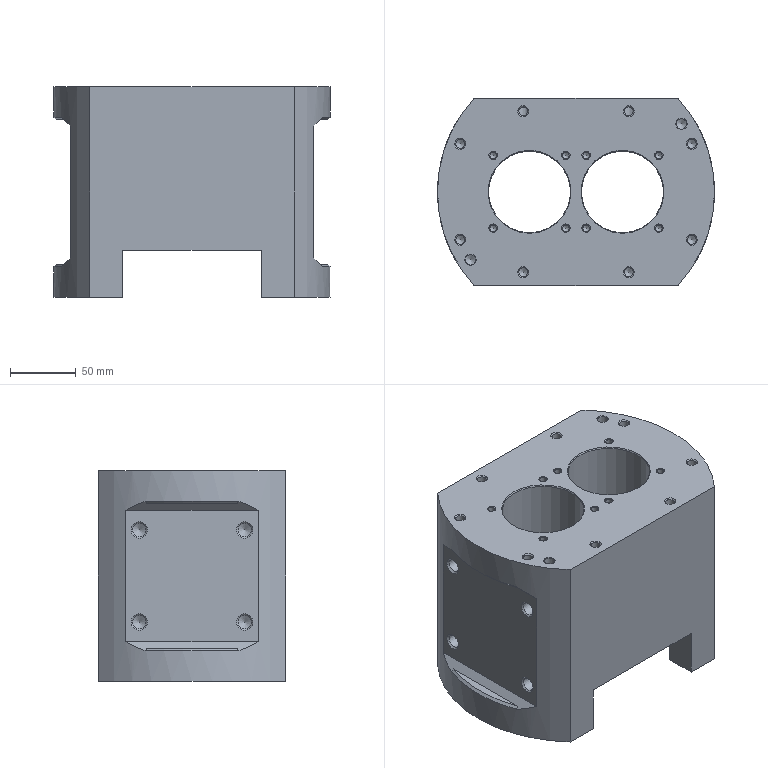NC program | NX | posted with a generic post | part box 210 x 142 x 160 mm
Lines 3328 to 4199 of 4199:
(FLOOR_WALL_2_COPY , TOOL : D10JING)
N6648 T11 M6
N6650 G54
N6652 G17 G0 G90 X-47.5 Y79. B0. C0. S5000 M3
N6654 G43 Z30. H11
N6656 Z-1.5
N6658 G94 G1 Z-4.5 F500.
N6660 Y76.
N6662 Y44.478 F1200.
N6664 X-50.809 Y43.289
N6666 G3 X-50.809 Y-43.289 R46.
N6668 G1 X-47.5 Y-44.478
N6670 Y-76.
N6672 Y-79.
N6674 Z-1.5
N6676 G0 Z30.
N6678 X47.5
N6680 Z-1.5
N6682 G1 Z-4.5 F500.
N6684 Y-76.
N6686 Y-44.478 F1200.
N6688 X50.809 Y-43.289
N6690 G3 X50.809 Y43.289 R46.
N6692 G1 X47.5 Y44.478
N6694 Y76.
N6696 Y79.
N6698 Z-1.5
N6700 G0 Z30.
N6702 X-47.5
N6704 Z-6.
N6706 G1 Z-9. F500.
N6708 Y76.
N6710 Y44.478 F1200.
N6712 X-50.809 Y43.289
N6714 G3 X-50.809 Y-43.289 R46.
N6716 G1 X-47.5 Y-44.478
N6718 Y-76.
N6720 Y-79.
N6722 Z-6.
N6724 G0 Z30.
N6726 X47.5
N6728 Z-6.
N6730 G1 Z-9. F500.
N6732 Y-76.
N6734 Y-44.478 F1200.
N6736 X50.809 Y-43.289
N6738 G3 X50.809 Y43.289 R46.
N6740 G1 X47.5 Y44.478
N6742 Y76.
N6744 Y79.
N6746 Z-6.
N6748 G0 Z30.
N6750 X-47.5
N6752 Z-10.5
N6754 G1 Z-13.5 F500.
N6756 Y76.
N6758 Y44.478 F1200.
N6760 X-50.809 Y43.289
N6762 G3 X-50.809 Y-43.289 R46.
N6764 G1 X-47.5 Y-44.478
N6766 Y-76.
N6768 Y-79.
N6770 Z-10.5
N6772 G0 Z30.
N6774 X47.5
N6776 Z-10.5
N6778 G1 Z-13.5 F500.
N6780 Y-76.
N6782 Y-44.478 F1200.
N6784 X50.809 Y-43.289
N6786 G3 X50.809 Y43.289 R46.
N6788 G1 X47.5 Y44.478
N6790 Y76.
N6792 Y79.
N6794 Z-10.5
N6796 G0 Z30.
N6798 X-47.5
N6800 Z-15.
N6802 G1 Z-18. F500.
N6804 Y76.
N6806 Y44.478 F1200.
N6808 X-50.809 Y43.289
N6810 G3 X-50.809 Y-43.289 R46.
N6812 G1 X-47.5 Y-44.478
N6814 Y-76.
N6816 Y-79.
N6818 Z-15.
N6820 G0 Z30.
N6822 X47.5
N6824 Z-15.
N6826 G1 Z-18. F500.
N6828 Y-76.
N6830 Y-44.478 F1200.
N6832 X50.809 Y-43.289
N6834 G3 X50.809 Y43.289 R46.
N6836 G1 X47.5 Y44.478
N6838 Y76.
N6840 Y79.
N6842 Z-15.
N6844 G0 Z30.
N6846 X-47.5
N6848 Z-19.5
N6850 G1 Z-22.5 F500.
N6852 Y76.
N6854 Y44.478 F1200.
N6856 X-50.809 Y43.289
N6858 G3 X-50.809 Y-43.289 R46.
N6860 G1 X-47.5 Y-44.478
N6862 Y-76.
N6864 Y-79.
N6866 Z-19.5
N6868 G0 Z30.
N6870 X47.5
N6872 Z-19.5
N6874 G1 Z-22.5 F500.
N6876 Y-76.
N6878 Y-44.478 F1200.
N6880 X50.809 Y-43.289
N6882 G3 X50.809 Y43.289 R46.
N6884 G1 X47.5 Y44.478
N6886 Y76.
N6888 Y79.
N6890 Z-19.5
N6892 G0 Z30.
N6894 X-47.5
N6896 Z-24.
N6898 G1 Z-27. F500.
N6900 Y76.
N6902 Y44.478 F1200.
N6904 X-50.809 Y43.289
N6906 G3 X-50.809 Y-43.289 R46.
N6908 G1 X-47.5 Y-44.478
N6910 Y-76.
N6912 Y-79.
N6914 Z-24.
N6916 G0 Z30.
N6918 X47.5
N6920 Z-24.
N6922 G1 Z-27. F500.
N6924 Y-76.
N6926 Y-44.478 F1200.
N6928 X50.809 Y-43.289
N6930 G3 X50.809 Y43.289 R46.
N6932 G1 X47.5 Y44.478
N6934 Y76.
N6936 Y79.
N6938 Z-24.
N6940 G0 Z30.
N6942 X-47.5
N6944 Z-28.5
N6946 G1 Z-31.5 F500.
N6948 Y76.
N6950 Y44.478 F1200.
N6952 X-50.809 Y43.289
N6954 G3 X-50.809 Y-43.289 R46.
N6956 G1 X-47.5 Y-44.478
N6958 Y-76.
N6960 Y-79.
N6962 Z-28.5
N6964 G0 Z30.
N6966 X47.5
N6968 Z-28.5
N6970 G1 Z-31.5 F500.
N6972 Y-76.
N6974 Y-44.478 F1200.
N6976 X50.809 Y-43.289
N6978 G3 X50.809 Y43.289 R46.
N6980 G1 X47.5 Y44.478
N6982 Y76.
N6984 Y79.
N6986 Z-28.5
N6988 G0 Z30.
N6990 X-47.5
N6992 Z-33.
N6994 G1 Z-36. F500.
N6996 Y76.
N6998 Y44.478 F1200.
N7000 X-50.809 Y43.289
N7002 G3 X-50.809 Y-43.289 R46.
N7004 G1 X-47.5 Y-44.478
N7006 Y-76.
N7008 Y-79.
N7010 Z-33.
N7012 G0 Z30.
N7014 X47.5
N7016 Z-33.
N7018 G1 Z-36. F500.
N7020 Y-76.
N7022 Y-44.478 F1200.
N7024 X50.809 Y-43.289
N7026 G3 X50.809 Y43.289 R46.
N7028 G1 X47.5 Y44.478
N7030 Y76.
N7032 Y79.
N7034 Z-33.
N7036 G0 Z30.
(FLOOR_WALL_2 , TOOL : D10JING)
N7038 X-80.75 Y-0.024
N7040 Z-30.
N7042 G95 G1 Y0.049 Z-30.019 F3.
N7044 Y-0.049 Z-30.046
N7046 Y0.049 Z-30.072
N7048 Y-0.049 Z-30.099
N7050 Y0.049 Z-30.125
N7052 Y-0.049 Z-30.151
N7054 Y0.049 Z-30.178
N7056 Y-0.049 Z-30.204
N7058 Y0.049 Z-30.23
N7060 Y-0.049 Z-30.257
N7062 Y0.049 Z-30.283
N7064 Y-0.049 Z-30.309
N7066 Y0.049 Z-30.336
N7068 Y-0.049 Z-30.362
N7070 Y0.049 Z-30.388
N7072 Y-0.049 Z-30.415
N7074 Y0.049 Z-30.441
N7076 Y-0.049 Z-30.467
N7078 Y0.049 Z-30.494
N7080 Y-0.049 Z-30.52
N7082 Y0.049 Z-30.546
N7084 Y-0.049 Z-30.573
N7086 Y0.049 Z-30.599
N7088 Y-0.049 Z-30.625
N7090 Y0.049 Z-30.652
N7092 Y-0.049 Z-30.678
N7094 Y0.049 Z-30.704
N7096 Y-0.049 Z-30.731
N7098 Y0.049 Z-30.757
N7100 Y-0.049 Z-30.784
N7102 Y0.049 Z-30.81
N7104 Y-0.049 Z-30.836
N7106 Y0.049 Z-30.863
N7108 Y-0.049 Z-30.889
N7110 Y0.049 Z-30.915
N7112 Y-0.049 Z-30.942
N7114 Y0.049 Z-30.968
N7116 Y-0.049 Z-30.994
N7118 Y0.049 Z-31.021
N7120 Y-0.049 Z-31.047
N7122 Y0.049 Z-31.073
N7124 Y-0.049 Z-31.1
N7126 Y0.049 Z-31.126
N7128 Y-0.049 Z-31.152
N7130 Y0.049 Z-31.179
N7132 Y-0.049 Z-31.205
N7134 Y0.049 Z-31.231
N7136 Y-0.049 Z-31.258
N7138 Y0.049 Z-31.284
N7140 Y-0.049 Z-31.31
N7142 Y0.049 Z-31.337
N7144 Y-0.049 Z-31.363
N7146 Y0.049 Z-31.389
N7148 Y-0.049 Z-31.416
N7150 Y0.049 Z-31.442
N7152 Y-0.049 Z-31.469
N7154 Y0.049 Z-31.495
N7156 Y-0.049 Z-31.521
N7158 Y0.049 Z-31.548
N7160 Y-0.049 Z-31.574
N7162 Y0.049 Z-31.6
N7164 Y-0.049 Z-31.627
N7166 Y0.049 Z-31.653
N7168 Y-0.049 Z-31.679
N7170 Y0.049 Z-31.706
N7172 Y-0.049 Z-31.732
N7174 Y0.049 Z-31.758
N7176 Y-0.049 Z-31.785
N7178 Y0.049 Z-31.811
N7180 Y-0.049 Z-31.837
N7182 Y0.049 Z-31.864
N7184 Y-0.049 Z-31.89
N7186 Y0.049 Z-31.916
N7188 Y-0.049 Z-31.943
N7190 Y0.049 Z-31.969
N7192 Y-0.049 Z-31.995
N7194 Y0.049 Z-32.022
N7196 Y-0.049 Z-32.048
N7198 Y0.049 Z-32.074
N7200 Y-0.049 Z-32.101
N7202 Y0.049 Z-32.127
N7204 Y-0.049 Z-32.154
N7206 Y0.049 Z-32.18
N7208 Y-0.049 Z-32.206
N7210 Y0.049 Z-32.233
N7212 Y-0.049 Z-32.259
N7214 Y0.049 Z-32.285
N7216 Y-0.049 Z-32.312
N7218 Y0.049 Z-32.338
N7220 Y-0.049 Z-32.364
N7222 Y0.049 Z-32.391
N7224 Y-0.049 Z-32.417
N7226 Y0.049 Z-32.443
N7228 Y-0.049 Z-32.47
N7230 Y0.049 Z-32.496
N7232 Y-0.049 Z-32.522
N7234 Y0.049 Z-32.549
N7236 Y-0.049 Z-32.575
N7238 Y0.049 Z-32.601
N7240 Y-0.049 Z-32.628
N7242 Y0.049 Z-32.654
N7244 Y-0.049 Z-32.68
N7246 Y0.049 Z-32.707
N7248 Y-0.049 Z-32.733
N7250 Y0.049 Z-32.759
N7252 Y-0.049 Z-32.786
N7254 Y0.049 Z-32.812
N7256 Y-0.049 Z-32.839
N7258 Y0.049 Z-32.865
N7260 Y-0.049 Z-32.891
N7262 Y0.049 Z-32.918
N7264 Y-0.049 Z-32.944
N7266 Y0.049 Z-32.97
N7268 Y-0.049 Z-32.997
N7270 Y0.049 Z-33.023
N7272 Y-0.049 Z-33.049
N7274 Y0.049 Z-33.076
N7276 Y-0.049 Z-33.102
N7278 Y0.049 Z-33.128
N7280 Y-0.049 Z-33.155
N7282 Y0.049 Z-33.181
N7284 Y-0.049 Z-33.207
N7286 Y0.049 Z-33.234
N7288 Y-0.049 Z-33.26
N7290 Y0.049 Z-33.286
N7292 Y-0.049 Z-33.313
N7294 Y0.049 Z-33.339
N7296 Y-0.049 Z-33.365
N7298 Y0.049 Z-33.392
N7300 Y-0.049 Z-33.418
N7302 Y0.049 Z-33.444
N7304 Y-0.049 Z-33.471
N7306 Y0.049 Z-33.497
N7308 Y-0.049 Z-33.523
N7310 Y0.049 Z-33.55
N7312 Y-0.049 Z-33.576
N7314 Y0.049 Z-33.603
N7316 Y-0.049 Z-33.629
N7318 Y0.049 Z-33.655
N7320 Y-0.049 Z-33.682
N7322 Y0.049 Z-33.708
N7324 Y-0.049 Z-33.734
N7326 Y0.049 Z-33.761
N7328 Y-0.049 Z-33.787
N7330 Y0.049 Z-33.813
N7332 Y-0.049 Z-33.84
N7334 Y0.049 Z-33.866
N7336 Y-0.049 Z-33.892
N7338 Y0.049 Z-33.919
N7340 Y-0.049 Z-33.945
N7342 Y0.049 Z-33.971
N7344 Y-0.049 Z-33.998
N7346 Y0.049 Z-34.024
N7348 Y-0.049 Z-34.05
N7350 Y0.049 Z-34.077
N7352 Y-0.049 Z-34.103
N7354 Y0.049 Z-34.129
N7356 Y-0.049 Z-34.156
N7358 Y0.049 Z-34.182
N7360 Y-0.049 Z-34.208
N7362 Y0.049 Z-34.235
N7364 Y-0.049 Z-34.261
N7366 Y0.049 Z-34.288
N7368 Y-0.049 Z-34.314
N7370 Y0.049 Z-34.34
N7372 Y-0.049 Z-34.367
N7374 Y0.049 Z-34.393
N7376 Y-0.049 Z-34.419
N7378 Y0.049 Z-34.446
N7380 Y-0.049 Z-34.472
N7382 Y0.049 Z-34.498
N7384 Y-0.049 Z-34.525
N7386 Y0.049 Z-34.551
N7388 Y-0.049 Z-34.577
N7390 Y0.049 Z-34.604
N7392 Y-0.049 Z-34.63
N7394 Y0.049 Z-34.656
N7396 Y-0.049 Z-34.683
N7398 Y0.049 Z-34.709
N7400 Y-0.049 Z-34.735
N7402 Y0.049 Z-34.762
N7404 Y-0.049 Z-34.788
N7406 Y0.049 Z-34.814
N7408 Y-0.049 Z-34.841
N7410 Y0.049 Z-34.867
N7412 Y-0.049 Z-34.893
N7414 Y0.049 Z-34.92
N7416 Y-0.049 Z-34.946
N7418 Y0.049 Z-34.973
N7420 Y-0.049 Z-34.999
N7422 Y0.049 Z-35.025
N7424 Y-0.049 Z-35.052
N7426 Y0.049 Z-35.078
N7428 Y-0.049 Z-35.104
N7430 Y0.049 Z-35.131
N7432 Y-0.049 Z-35.157
N7434 Y0.049 Z-35.183
N7436 Y-0.049 Z-35.21
N7438 Y0.049 Z-35.236
N7440 Y-0.049 Z-35.262
N7442 Y0.049 Z-35.289
N7444 Y-0.049 Z-35.315
N7446 Y0.049 Z-35.341
N7448 Y-0.049 Z-35.368
N7450 Y0.049 Z-35.394
N7452 Y-0.049 Z-35.42
N7454 Y0.049 Z-35.447
N7456 Y-0.049 Z-35.473
N7458 Y0.049 Z-35.499
N7460 Y-0.049 Z-35.526
N7462 Y0.049 Z-35.552
N7464 Y-0.049 Z-35.578
N7466 Y0.049 Z-35.605
N7468 Y-0.049 Z-35.631
N7470 Y0.049 Z-35.658
N7472 Y-0.049 Z-35.684
N7474 Y0.049 Z-35.71
N7476 Y-0.049 Z-35.737
N7478 Y0.049 Z-35.763
N7480 Y-0.049 Z-35.789
N7482 Y0.049 Z-35.816
N7484 Y-0.049 Z-35.842
N7486 Y0.049 Z-35.868
N7488 Y-0.049 Z-35.895
N7490 Y0.049 Z-35.921
N7492 Y-0.049 Z-35.947
N7494 Y0.049 Z-35.974
N7496 Y-0.049 Z-36.
N7498 G94 Y0.049 F1200.
N7500 G2 X-75.856 Y20.528 R45.5
N7502 G1 Y-20.528
N7504 G3 X-70.962 Y-28.194 R45.5
N7506 G1 Y28.194
N7508 G2 X-66.068 Y33.474 R45.5
N7510 G1 Y-33.474
N7512 G3 X-61.174 Y-37.392 R45.5
N7514 G1 Y37.392
N7516 G2 X-56.28 Y40.348 R45.5
N7518 G1 Y-40.348
N7520 G3 X-51.386 Y-42.543 R45.5
N7522 G1 Y42.543
N7524 G2 X-50.64 Y42.818 R45.5
N7526 G1 X-47.331 Y44.008
N7528 G3 X-47. Y44.478 R0.5
N7530 G1 Y76.
N7532 X-46.492
N7534 Y-76.
N7536 X-41.598
N7538 Y76.
N7540 X-36.705
N7542 Y-76.
N7544 X-31.811
N7546 Y76.
N7548 X-26.917
N7550 Y-76.
N7552 X-22.023
N7554 Y76.
N7556 X-17.129
N7558 Y-76.
N7560 X-12.235
N7562 Y76.
N7564 X-7.341
N7566 Y-76.
N7568 X-2.447
N7570 Y76.
N7572 X2.447
N7574 Y-76.
N7576 X7.341
N7578 Y76.
N7580 X12.235
N7582 Y-76.
N7584 X17.129
N7586 Y76.
N7588 X22.023
N7590 Y-76.
N7592 X26.917
N7594 Y76.
N7596 X31.811
N7598 Y-76.
N7600 X36.705
N7602 Y76.
N7604 X41.598
N7606 Y-76.
N7608 X46.492
N7610 Y76.
N7612 X47.
N7614 Y44.478
N7616 G3 X47.331 Y44.008 R0.5
N7618 G1 X50.64 Y42.818
N7620 G2 X51.386 Y42.543 R45.5
N7622 G1 Y-42.543
N7624 G3 X56.28 Y-40.348 R45.5
N7626 G1 Y40.348
N7628 G2 X61.174 Y37.392 R45.5
N7630 G1 Y-37.392
N7632 G3 X66.068 Y-33.474 R45.5
N7634 G1 Y33.474
N7636 G2 X70.962 Y28.194 R45.5
N7638 G1 Y-28.194
N7640 G3 X75.856 Y-20.528 R45.5
N7642 G1 Y20.528
N7644 G2 X80.75 Y0.049 R45.5
N7646 G1 Y-0.049
N7648 Z-33.
N7650 G0 Z30.
N7652 X47.5 Y-79.
N7654 Z-33.
N7656 G95 G1 Z-36. F3.
N7658 Y-76.
N7660 G94 Y-44.478 F1200.
N7662 X50.809 Y-43.289
N7664 G3 X50.809 Y43.289 R46.
N7666 G1 X47.5 Y44.478
N7668 Y76.
N7670 Y79.
N7672 Z-33.
N7674 G0 Z30.
N7676 X-47.5
N7678 Z-33.
N7680 G95 G1 Z-36. F3.
N7682 Y76.
N7684 G94 Y44.478 F1200.
N7686 X-50.809 Y43.289
N7688 G3 X-50.809 Y-43.289 R46.
N7690 G1 X-47.5 Y-44.478
N7692 Y-76.
N7694 Y-79.
N7696 Z-33.
N7698 G0 Z30.
N7700 M5
(DRILLING_COPY_2_COPY_1 , TOOL : ZXZ)
N7702 T01 M6
N7704 G54
N7706 G17 G0 G90 X69. Y59. B0. C0. S5000 M3
N7708 G43 Z30. H1
N7710 G94 G81 G98 Z-1. F250. R3.
N7712 X82. Y47.
N7714 X62.827 Y27.577 Z-37. R-33.
N7716 X7.673
N7718 X-7.673
N7720 Y-27.577
N7722 X7.673
N7724 X35.25 Y0.
N7726 X62.827 Y-27.577
N7728 X69. Y-59. Z-1. R3.
N7730 X-69.
N7732 X-82. Y-47.
N7734 X-62.827 Y-27.577 Z-37. R-33.
N7736 X-35.25 Y0.
N7738 X-62.827 Y27.577
N7740 X-69. Y59. Z-1. R3.
N7742 G80
N7744 G0 X-69. Y59. Z30.
N7746 M5
(DRILLING_COPY_2_COPY_COPY_1_COPY_2 , TOOL : 5.2ZT)
N7748 T15 M6
N7750 G54
N7752 G17 G0 G90 X-62.827 Y-27.577 B0. C0. S2000 M3
N7754 G43 Z30. H15
N7756 G94 G83 G98 Z-57.502 F200. Q2. R-33.
N7758 Y27.577
N7760 X-7.673
N7762 X7.673
N7764 X62.827
N7766 Y-27.577
N7768 X7.673
N7770 X-7.673
N7772 G80
N7774 G0 X-7.673 Y-27.577 Z30.
N7776 M5
(DRILLING_COPY_2_COPY_COPY_1_COPY_2_COPY , TOOL : 8.5ZT)
N7778 T20 M6
N7780 G54
N7782 G17 G0 G90 X-69. Y-59. B0. C0. S2000 M3
N7784 G43 Z30. H20
N7786 G94 G83 G98 Z-32.054 F200. Q2. R3.
N7788 Y59.
N7790 X69.
N7792 Y-59.
N7794 G80
N7796 G0 X69. Y-59. Z30.
N7798 M5
(DRILLING_COPY_2_COPY_COPY_1_COPY_1_COPY_1 , TOOL : 9.8ZT)
N7800 T03 M6
N7802 G54
N7804 G17 G0 G90 X82. Y47. B0. C0. S2000 M3
N7806 G43 Z30. H3
N7808 G94 G83 G98 Z-23.004 F200. Q2. R3.
N7810 X-82. Y-47.
N7812 G80
N7814 G0 X-82. Y-47. Z30.
N7816 M5
(DRILLING_COPY_2_COPY_COPY_1_COPY_1_COPY_COPY_1 , TOOL : 10.JD)
N7818 T04 M6
N7820 G54
N7822 G17 G0 G90 X-82. Y-47. B0. C0. S1000 M3
N7824 G43 Z30. H4
N7826 G94 G85 G98 Z-20. F40. R3.
N7828 X82. Y47.
N7830 G80
N7832 G0 X82. Y47. Z30.
N7834 M5
(PLANAR_MILL_COPY_COPY_COPY_COPY_COPY_1 , TOOL : D6A45)
N7836 T07 M6
N7838 G54
N7840 G17 G0 G90 X-68.438 Y61.487 B0. C0. S7500 M3
N7842 G43 Z30. H7
N7844 Z1.5
N7846 G94 G1 Z-1.5 F1250.
N7848 X-68.234 Y62.393
N7850 G3 X-69. Y62.75 R1.
N7852 X-72.75 Y59. R3.75
N7854 X-69. Y62.75 R-3.75
N7856 X-69.766 Y62.393 R1.
N7858 G1 X-69.562 Y61.487
N7860 Z1.5
N7862 G0 Z30.
N7864 X-84.487 Y-46.438
N7866 Z1.5
N7868 G1 Z-1.5
N7870 X-85.393 Y-46.234
N7872 G3 X-85.75 Y-47. R1.
N7874 X-82. Y-50.75 R3.75
N7876 X-85.75 Y-47. R-3.75
N7878 X-85.393 Y-47.766 R1.
N7880 G1 X-84.487 Y-47.562
N7882 Z1.5
N7884 G0 Z30.
N7886 X-69.562 Y-61.487
N7888 Z1.5
N7890 G1 Z-1.5
N7892 X-69.766 Y-62.393
N7894 G3 X-69. Y-62.75 R1.
N7896 X-65.25 Y-59. R3.75
N7898 X-69. Y-62.75 R-3.75
N7900 X-68.234 Y-62.393 R1.
N7902 G1 X-68.438 Y-61.487
N7904 Z1.5
N7906 G0 Z30.
N7908 X68.438
N7910 Z1.5
N7912 G1 Z-1.5
N7914 X68.234 Y-62.393
N7916 G3 X69. Y-62.75 R1.
N7918 X72.75 Y-59. R3.75
N7920 X69. Y-62.75 R-3.75
N7922 X69.766 Y-62.393 R1.
N7924 G1 X69.562 Y-61.487
N7926 Z1.5
N7928 G0 Z30.
N7930 X84.487 Y46.438
N7932 Z1.5
N7934 G1 Z-1.5
N7936 X85.393 Y46.234
N7938 G3 X85.75 Y47. R1.
N7940 X82. Y50.75 R3.75
N7942 X85.75 Y47. R-3.75
N7944 X85.393 Y47.766 R1.
N7946 G1 X84.487 Y47.562
N7948 Z1.5
N7950 G0 Z30.
N7952 X69.562 Y61.487
N7954 Z1.5
N7956 G1 Z-1.5
N7958 X69.766 Y62.393
N7960 G3 X69. Y62.75 R1.
N7962 X65.25 Y59. R3.75
N7964 X69. Y62.75 R-3.75
N7966 X68.234 Y62.393 R1.
N7968 G1 X68.438 Y61.487
N7970 Z1.5
N7972 G0 Z30.
(PLANAR_MILL_COPY_COPY_COPY_COPY_COPY_1_COPY , TOOL : D6A45)
N7974 X63.309 Y-27.842
N7976 Z-34.5
N7978 G1 Z-37.5
N7980 X64.22 Y-28.343
N7982 G3 X64.577 Y-27.577 R1.
N7984 X62.827 Y-25.827 R1.75
N7986 X64.577 Y-27.577 R-1.75
N7988 X64.22 Y-26.811 R1.
N7990 G1 X63.309 Y-27.312
N7992 Z-34.5
N7994 G0 Z30.
N7996 X7.408 Y-28.059
N7998 Z-34.5
N8000 G1 Z-37.5
N8002 X6.907 Y-28.97
N8004 G3 X7.673 Y-29.327 R1.
N8006 X9.423 Y-27.577 R1.75
N8008 X7.673 Y-29.327 R-1.75
N8010 X8.439 Y-28.97 R1.
N8012 G1 X7.938 Y-28.059
N8014 Z-34.5
N8016 G0 Z30.
N8018 X-7.938
N8020 Z-34.5
N8022 G1 Z-37.5
N8024 X-8.439 Y-28.97
N8026 G3 X-7.673 Y-29.327 R1.
N8028 X-5.923 Y-27.577 R1.75
N8030 X-7.673 Y-29.327 R-1.75
N8032 X-6.907 Y-28.97 R1.
N8034 G1 X-7.408 Y-28.059
N8036 Z-34.5
N8038 G0 Z30.
N8040 X-63.309 Y-27.312
N8042 Z-34.5
N8044 G1 Z-37.5
N8046 X-64.22 Y-26.811
N8048 G3 X-64.577 Y-27.577 R1.
N8050 X-62.827 Y-29.327 R1.75
N8052 X-64.577 Y-27.577 R-1.75
N8054 X-64.22 Y-28.343 R1.
N8056 G1 X-63.309 Y-27.842
N8058 Z-34.5
N8060 G0 Z30.
N8062 Y27.842
N8064 Z-34.5
N8066 G1 Z-37.5
N8068 X-64.22 Y28.343
N8070 G3 X-64.577 Y27.577 R1.
N8072 X-62.827 Y25.827 R1.75
N8074 X-64.577 Y27.577 R-1.75
N8076 X-64.22 Y26.811 R1.
N8078 G1 X-63.309 Y27.312
N8080 Z-34.5
N8082 G0 Z30.
N8084 X-63.977 Y1.506
N8086 Z-34.5
N8088 G1 Z-37.5
N8090 X-64.859 Y0.766
N8092 G3 X-65.216 Y0. R1.
N8094 X-35.25 Y-29.966 R29.966
N8096 X-65.216 Y0. R-29.966
N8098 X-64.859 Y-0.766 R1.
N8100 G1 X-63.977 Y-1.506
N8102 Z-34.5
N8104 G0 Z30.
N8106 X-7.408 Y28.059
N8108 Z-34.5
N8110 G1 Z-37.5
N8112 X-6.907 Y28.97
N8114 G3 X-7.673 Y29.327 R1.
N8116 X-9.423 Y27.577 R1.75
N8118 X-7.673 Y29.327 R-1.75
N8120 X-8.439 Y28.97 R1.
N8122 G1 X-7.938 Y28.059
N8124 Z-34.5
N8126 G0 Z30.
N8128 X7.938
N8130 Z-34.5
N8132 G1 Z-37.5
N8134 X8.439 Y28.97
N8136 G3 X7.673 Y29.327 R1.
N8138 X5.923 Y27.577 R1.75
N8140 X7.673 Y29.327 R-1.75
N8142 X6.907 Y28.97 R1.
N8144 G1 X7.408 Y28.059
N8146 Z-34.5
N8148 G0 Z30.
N8150 X63.977 Y-1.506
N8152 Z-34.5
N8154 G1 Z-37.5
N8156 X64.859 Y-0.766
N8158 G3 X65.216 Y0. R1.
N8160 X35.25 Y29.966 R29.966
N8162 X65.216 Y0. R-29.966
N8164 X64.859 Y0.766 R1.
N8166 G1 X63.977 Y1.506
N8168 Z-34.5
N8170 G0 Z30.
N8172 X63.309 Y27.312
N8174 Z-34.5
N8176 G1 Z-37.5
N8178 X64.22 Y26.811
N8180 G3 X64.577 Y27.577 R1.
N8182 X62.827 Y29.327 R1.75
N8184 X64.577 Y27.577 R-1.75
N8186 X64.22 Y28.343 R1.
N8188 G1 X63.309 Y27.842
N8190 Z-34.5
N8192 G0 Z30.
(PLANAR_MILL_COPY_COPY_COPY_COPY_COPY_COPY , TOOL : D6A45)
N8194 X63.511 Y73.5
N8196 Z1.5
N8198 G1 Z-1.5
N8200 X64.218 Y72.657
N8202 G3 X64.984 Y72.3 R1.
N8204 G1 X77.268
N8206 G2 X78.374 Y71.813 R1.5
N8208 X78.374 Y-71.813 R106.3
N8210 X77.268 Y-72.3 R1.5
N8212 G1 X52.7
N8214 G2 X51.2 Y-70.8 R1.5
N8216 G1 Y-48.135
N8218 G2 X52.189 Y-46.724 R1.5
N8220 G3 X52.189 Y46.724 R49.7
N8222 G2 X51.2 Y48.135 R1.5
N8224 G1 Y70.8
N8226 G2 X52.7 Y72.3 R1.5
N8228 G1 X64.984
N8230 G3 X65.75 Y72.657 R1.
N8232 G1 X66.457 Y73.5
N8234 Z1.5
N8236 G0 Z30.
N8238 X-66.457
N8240 Z1.5
N8242 G1 Z-1.5
N8244 X-65.75 Y72.657
N8246 G3 X-64.984 Y72.3 R1.
N8248 G1 X-52.7
N8250 G2 X-51.2 Y70.8 R1.5
N8252 G1 Y48.135
N8254 G2 X-52.189 Y46.724 R1.5
N8256 G3 X-52.189 Y-46.724 R49.7
N8258 G2 X-51.2 Y-48.135 R1.5
N8260 G1 Y-70.8
N8262 G2 X-52.7 Y-72.3 R1.5
N8264 G1 X-77.268
N8266 G2 X-78.374 Y-71.813 R1.5
N8268 X-78.374 Y71.813 R106.3
N8270 X-77.268 Y72.3 R1.5
N8272 G1 X-64.984
N8274 G3 X-64.218 Y72.657 R1.
N8276 G1 X-63.511 Y73.5
N8278 Z1.5
N8280 G0 Z30.
(PLANAR_MILL_COPY_COPY_COPY_COPY_COPY_COPY_COPY , TOOL : D6A45)
N8282 X-48.799 Y73.897
N8284 Z-34.5
N8286 G1 Z-37.5
N8288 X-49.203 Y73.144
N8290 G3 X-49.25 Y72.3 R1.
N8292 G1 X49.25
N8294 G3 X49.203 Y73.144 R1.
N8296 G1 X48.799 Y73.897
N8298 Z-34.5
N8300 G0 Z30.
N8302 Y-73.897
N8304 Z-34.5
N8306 G1 Z-37.5
N8308 X49.203 Y-73.144
N8310 G3 X49.25 Y-72.3 R1.
N8312 G1 X-49.25
N8314 G3 X-49.203 Y-73.144 R1.
N8316 G1 X-48.799 Y-73.897
N8318 Z-34.5
N8320 G0 Z30.
N8322 M5
N8324 M2